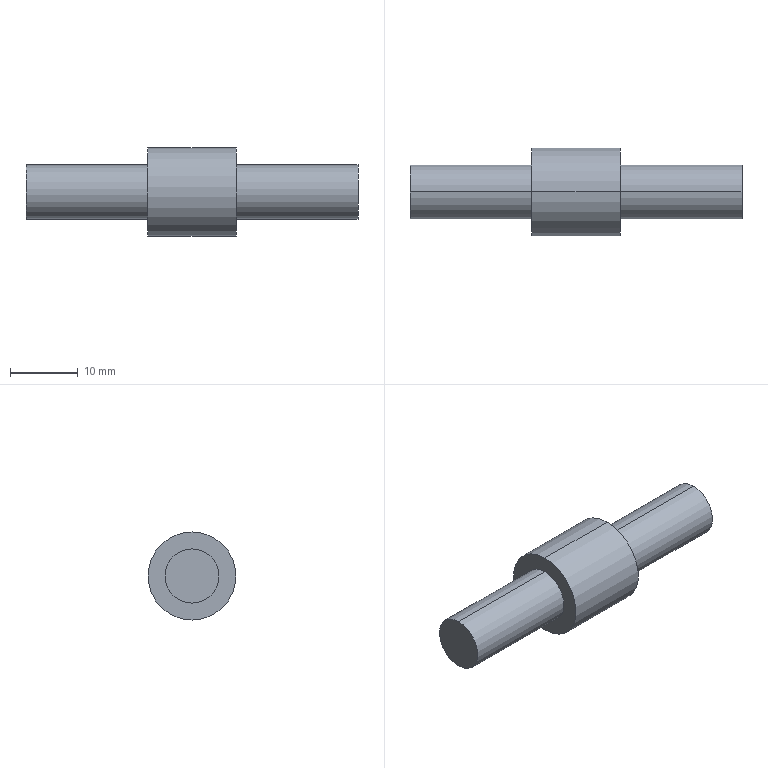Part | SolidWorks | features Extrusion 1, ICE 1, MirrorPattern 1 | 1 solid | 10 faces | box 49 x 13 x 13 mm | volume 3535 mm3 | cylinder 6 | plane 4 | commonest cylinder face diameters 8 x4 13 x2
STEP:
#1=CARTESIAN_POINT('',(-24.5,0.,-4.));
#2=VERTEX_POINT('',#1);
#3=CARTESIAN_POINT('',(-24.5,0.,4.));
#4=VERTEX_POINT('',#3);
#5=CARTESIAN_POINT('',(-24.5,0.,0.));
#6=DIRECTION('',(1.,0.,0.));
#7=DIRECTION('',(0.,0.,-1.));
#8=AXIS2_PLACEMENT_3D('',#5,#6,#7);
#9=CIRCLE('',#8,4.);
#10=EDGE_CURVE('',#2,#4,#9,.T.);
#11=ORIENTED_EDGE('',*,*,#10,.T.);
#12=CARTESIAN_POINT('',(-6.5,0.,4.));
#13=VERTEX_POINT('',#12);
#14=CARTESIAN_POINT('',(-24.5,0.,4.));
#15=DIRECTION('',(1.,0.,0.));
#16=VECTOR('',#15,1000.);
#17=LINE('',#14,#16);
#18=EDGE_CURVE('',#4,#13,#17,.T.);
#19=ORIENTED_EDGE('',*,*,#18,.T.);
#20=CARTESIAN_POINT('',(-6.5,0.,-4.));
#21=VERTEX_POINT('',#20);
#22=CARTESIAN_POINT('',(-6.5,0.,0.));
#23=DIRECTION('',(1.,0.,0.));
#24=DIRECTION('',(0.,0.,-1.));
#25=AXIS2_PLACEMENT_3D('',#22,#23,#24);
#26=CIRCLE('',#25,4.);
#27=EDGE_CURVE('',#21,#13,#26,.T.);
#28=ORIENTED_EDGE('',*,*,#27,.F.);
#29=CARTESIAN_POINT('',(-24.5,0.,-4.));
#30=DIRECTION('',(1.,0.,0.));
#31=VECTOR('',#30,1000.);
#32=LINE('',#29,#31);
#33=EDGE_CURVE('',#2,#21,#32,.T.);
#34=ORIENTED_EDGE('',*,*,#33,.F.);
#35=EDGE_LOOP('',(#11,#19,#28,#34));
#36=FACE_OUTER_BOUND('',#35,.T.);
#37=CARTESIAN_POINT('',(-24.5,0.,0.));
#38=DIRECTION('',(1.,0.,0.));
#39=DIRECTION('',(0.,0.,-1.));
#40=AXIS2_PLACEMENT_3D('',#37,#38,#39);
#41=CYLINDRICAL_SURFACE('',#40,4.);
#42=ADVANCED_FACE('',(#36),#41,.T.);
#43=CARTESIAN_POINT('',(24.5,0.,-4.));
#44=VERTEX_POINT('',#43);
#45=CARTESIAN_POINT('',(24.5,0.,4.));
#46=VERTEX_POINT('',#45);
#47=CARTESIAN_POINT('',(24.5,0.,0.));
#48=DIRECTION('',(1.,0.,0.));
#49=DIRECTION('',(0.,0.,-1.));
#50=AXIS2_PLACEMENT_3D('',#47,#48,#49);
#51=CIRCLE('',#50,4.);
#52=EDGE_CURVE('',#44,#46,#51,.T.);
#53=ORIENTED_EDGE('',*,*,#52,.F.);
#54=CARTESIAN_POINT('',(6.5,0.,-4.));
#55=VERTEX_POINT('',#54);
#56=CARTESIAN_POINT('',(24.5,0.,-4.));
#57=DIRECTION('',(-1.,0.,0.));
#58=VECTOR('',#57,1000.);
#59=LINE('',#56,#58);
#60=EDGE_CURVE('',#44,#55,#59,.T.);
#61=ORIENTED_EDGE('',*,*,#60,.T.);
#62=CARTESIAN_POINT('',(6.5,0.,4.));
#63=VERTEX_POINT('',#62);
#64=CARTESIAN_POINT('',(6.5,0.,0.));
#65=DIRECTION('',(1.,0.,0.));
#66=DIRECTION('',(0.,0.,-1.));
#67=AXIS2_PLACEMENT_3D('',#64,#65,#66);
#68=CIRCLE('',#67,4.);
#69=EDGE_CURVE('',#55,#63,#68,.T.);
#70=ORIENTED_EDGE('',*,*,#69,.T.);
#71=CARTESIAN_POINT('',(24.5,0.,4.));
#72=DIRECTION('',(-1.,0.,0.));
#73=VECTOR('',#72,1000.);
#74=LINE('',#71,#73);
#75=EDGE_CURVE('',#46,#63,#74,.T.);
#76=ORIENTED_EDGE('',*,*,#75,.F.);
#77=EDGE_LOOP('',(#53,#61,#70,#76));
#78=FACE_OUTER_BOUND('',#77,.T.);
#79=CARTESIAN_POINT('',(24.5,0.,0.));
#80=DIRECTION('',(-1.,0.,0.));
#81=DIRECTION('',(0.,0.,1.));
#82=AXIS2_PLACEMENT_3D('',#79,#80,#81);
#83=CYLINDRICAL_SURFACE('',#82,4.);
#84=ADVANCED_FACE('',(#78),#83,.T.);
#85=CARTESIAN_POINT('',(6.5,0.,-6.5));
#86=VERTEX_POINT('',#85);
#87=CARTESIAN_POINT('',(6.5,0.,6.5));
#88=VERTEX_POINT('',#87);
#89=CARTESIAN_POINT('',(6.5,0.,0.));
#90=DIRECTION('',(1.,0.,0.));
#91=DIRECTION('',(0.,0.,-1.));
#92=AXIS2_PLACEMENT_3D('',#89,#90,#91);
#93=CIRCLE('',#92,6.5);
#94=EDGE_CURVE('',#86,#88,#93,.T.);
#95=ORIENTED_EDGE('',*,*,#94,.F.);
#96=CARTESIAN_POINT('',(-6.5,0.,-6.5));
#97=VERTEX_POINT('',#96);
#98=CARTESIAN_POINT('',(6.5,0.,-6.5));
#99=DIRECTION('',(-1.,0.,0.));
#100=VECTOR('',#99,1000.);
#101=LINE('',#98,#100);
#102=EDGE_CURVE('',#86,#97,#101,.T.);
#103=ORIENTED_EDGE('',*,*,#102,.T.);
#104=CARTESIAN_POINT('',(-6.5,0.,6.5));
#105=VERTEX_POINT('',#104);
#106=CARTESIAN_POINT('',(-6.5,0.,0.));
#107=DIRECTION('',(1.,0.,0.));
#108=DIRECTION('',(0.,0.,-1.));
#109=AXIS2_PLACEMENT_3D('',#106,#107,#108);
#110=CIRCLE('',#109,6.5);
#111=EDGE_CURVE('',#97,#105,#110,.T.);
#112=ORIENTED_EDGE('',*,*,#111,.T.);
#113=CARTESIAN_POINT('',(6.5,0.,6.5));
#114=DIRECTION('',(-1.,0.,0.));
#115=VECTOR('',#114,1000.);
#116=LINE('',#113,#115);
#117=EDGE_CURVE('',#88,#105,#116,.T.);
#118=ORIENTED_EDGE('',*,*,#117,.F.);
#119=EDGE_LOOP('',(#95,#103,#112,#118));
#120=FACE_OUTER_BOUND('',#119,.T.);
#121=CARTESIAN_POINT('',(6.5,0.,0.));
#122=DIRECTION('',(-1.,0.,0.));
#123=DIRECTION('',(0.,0.,1.));
#124=AXIS2_PLACEMENT_3D('',#121,#122,#123);
#125=CYLINDRICAL_SURFACE('',#124,6.5);
#126=ADVANCED_FACE('',(#120),#125,.T.);
#127=ORIENTED_EDGE('',*,*,#102,.F.);
#128=CARTESIAN_POINT('',(6.5,0.,0.));
#129=DIRECTION('',(1.,0.,0.));
#130=DIRECTION('',(0.,0.,-1.));
#131=AXIS2_PLACEMENT_3D('',#128,#129,#130);
#132=CIRCLE('',#131,6.5);
#133=EDGE_CURVE('',#88,#86,#132,.T.);
#134=ORIENTED_EDGE('',*,*,#133,.F.);
#135=ORIENTED_EDGE('',*,*,#117,.T.);
#136=CARTESIAN_POINT('',(-6.5,0.,0.));
#137=DIRECTION('',(1.,0.,0.));
#138=DIRECTION('',(0.,0.,-1.));
#139=AXIS2_PLACEMENT_3D('',#136,#137,#138);
#140=CIRCLE('',#139,6.5);
#141=EDGE_CURVE('',#105,#97,#140,.T.);
#142=ORIENTED_EDGE('',*,*,#141,.T.);
#143=EDGE_LOOP('',(#127,#134,#135,#142));
#144=FACE_OUTER_BOUND('',#143,.T.);
#145=CARTESIAN_POINT('',(6.5,0.,0.));
#146=DIRECTION('',(-1.,0.,0.));
#147=DIRECTION('',(0.,0.,1.));
#148=AXIS2_PLACEMENT_3D('',#145,#146,#147);
#149=CYLINDRICAL_SURFACE('',#148,6.5);
#150=ADVANCED_FACE('',(#144),#149,.T.);
#151=CARTESIAN_POINT('',(6.5,0.,0.));
#152=DIRECTION('',(1.,0.,0.));
#153=DIRECTION('',(0.,0.,-1.));
#154=AXIS2_PLACEMENT_3D('',#151,#152,#153);
#155=CIRCLE('',#154,4.);
#156=EDGE_CURVE('',#63,#55,#155,.T.);
#157=ORIENTED_EDGE('',*,*,#156,.F.);
#158=ORIENTED_EDGE('',*,*,#69,.F.);
#159=EDGE_LOOP('',(#157,#158));
#160=FACE_BOUND('',#159,.T.);
#161=ORIENTED_EDGE('',*,*,#133,.T.);
#162=ORIENTED_EDGE('',*,*,#94,.T.);
#163=EDGE_LOOP('',(#161,#162));
#164=FACE_OUTER_BOUND('',#163,.T.);
#165=CARTESIAN_POINT('',(6.5,0.,0.));
#166=DIRECTION('',(1.,0.,0.));
#167=DIRECTION('',(0.,0.,-1.));
#168=AXIS2_PLACEMENT_3D('',#165,#166,#167);
#169=PLANE('',#168);
#170=ADVANCED_FACE('',(#160,#164),#169,.T.);
#171=ORIENTED_EDGE('',*,*,#27,.T.);
#172=CARTESIAN_POINT('',(-6.5,0.,0.));
#173=DIRECTION('',(1.,0.,0.));
#174=DIRECTION('',(0.,0.,-1.));
#175=AXIS2_PLACEMENT_3D('',#172,#173,#174);
#176=CIRCLE('',#175,4.);
#177=EDGE_CURVE('',#13,#21,#176,.T.);
#178=ORIENTED_EDGE('',*,*,#177,.T.);
#179=EDGE_LOOP('',(#171,#178));
#180=FACE_BOUND('',#179,.T.);
#181=ORIENTED_EDGE('',*,*,#141,.F.);
#182=ORIENTED_EDGE('',*,*,#111,.F.);
#183=EDGE_LOOP('',(#181,#182));
#184=FACE_OUTER_BOUND('',#183,.T.);
#185=CARTESIAN_POINT('',(-6.5,0.,0.));
#186=DIRECTION('',(1.,0.,0.));
#187=DIRECTION('',(0.,0.,-1.));
#188=AXIS2_PLACEMENT_3D('',#185,#186,#187);
#189=PLANE('',#188);
#190=ADVANCED_FACE('',(#180,#184),#189,.F.);
#191=ORIENTED_EDGE('',*,*,#60,.F.);
#192=CARTESIAN_POINT('',(24.5,0.,0.));
#193=DIRECTION('',(1.,0.,0.));
#194=DIRECTION('',(0.,0.,-1.));
#195=AXIS2_PLACEMENT_3D('',#192,#193,#194);
#196=CIRCLE('',#195,4.);
#197=EDGE_CURVE('',#46,#44,#196,.T.);
#198=ORIENTED_EDGE('',*,*,#197,.F.);
#199=ORIENTED_EDGE('',*,*,#75,.T.);
#200=ORIENTED_EDGE('',*,*,#156,.T.);
#201=EDGE_LOOP('',(#191,#198,#199,#200));
#202=FACE_OUTER_BOUND('',#201,.T.);
#203=CARTESIAN_POINT('',(24.5,0.,0.));
#204=DIRECTION('',(-1.,0.,0.));
#205=DIRECTION('',(0.,0.,1.));
#206=AXIS2_PLACEMENT_3D('',#203,#204,#205);
#207=CYLINDRICAL_SURFACE('',#206,4.);
#208=ADVANCED_FACE('',(#202),#207,.T.);
#209=ORIENTED_EDGE('',*,*,#197,.T.);
#210=ORIENTED_EDGE('',*,*,#52,.T.);
#211=EDGE_LOOP('',(#209,#210));
#212=FACE_OUTER_BOUND('',#211,.T.);
#213=CARTESIAN_POINT('',(24.5,0.,0.));
#214=DIRECTION('',(1.,0.,0.));
#215=DIRECTION('',(0.,0.,-1.));
#216=AXIS2_PLACEMENT_3D('',#213,#214,#215);
#217=PLANE('',#216);
#218=ADVANCED_FACE('',(#212),#217,.T.);
#219=ORIENTED_EDGE('',*,*,#18,.F.);
#220=CARTESIAN_POINT('',(-24.5,0.,0.));
#221=DIRECTION('',(1.,0.,0.));
#222=DIRECTION('',(0.,0.,-1.));
#223=AXIS2_PLACEMENT_3D('',#220,#221,#222);
#224=CIRCLE('',#223,4.);
#225=EDGE_CURVE('',#4,#2,#224,.T.);
#226=ORIENTED_EDGE('',*,*,#225,.T.);
#227=ORIENTED_EDGE('',*,*,#33,.T.);
#228=ORIENTED_EDGE('',*,*,#177,.F.);
#229=EDGE_LOOP('',(#219,#226,#227,#228));
#230=FACE_OUTER_BOUND('',#229,.T.);
#231=CARTESIAN_POINT('',(-24.5,0.,0.));
#232=DIRECTION('',(1.,0.,0.));
#233=DIRECTION('',(0.,0.,-1.));
#234=AXIS2_PLACEMENT_3D('',#231,#232,#233);
#235=CYLINDRICAL_SURFACE('',#234,4.);
#236=ADVANCED_FACE('',(#230),#235,.T.);
#237=ORIENTED_EDGE('',*,*,#10,.F.);
#238=ORIENTED_EDGE('',*,*,#225,.F.);
#239=EDGE_LOOP('',(#237,#238));
#240=FACE_OUTER_BOUND('',#239,.T.);
#241=CARTESIAN_POINT('',(-24.5,0.,0.));
#242=DIRECTION('',(-1.,0.,0.));
#243=DIRECTION('',(0.,0.,-1.));
#244=AXIS2_PLACEMENT_3D('',#241,#242,#243);
#245=PLANE('',#244);
#246=ADVANCED_FACE('',(#240),#245,.T.);
#247=CLOSED_SHELL('',(#42,#84,#126,#150,#170,#190,#208,#218,#236,#246));
#248=MANIFOLD_SOLID_BREP('',#247);
#249=CARTESIAN_POINT('',(0.,0.,0.));
#250=DIRECTION('',(0.,0.,1.));
#251=DIRECTION('',(1.,0.,0.));
#252=AXIS2_PLACEMENT_3D('',#249,#250,#251);
#253=(LENGTH_UNIT()NAMED_UNIT(*)SI_UNIT(.MILLI.,.METRE.));
#254=UNCERTAINTY_MEASURE_WITH_UNIT(LENGTH_MEASURE(0.00001),#253,'','');
#255=(NAMED_UNIT(*)PLANE_ANGLE_UNIT()SI_UNIT($,.RADIAN.));
#256=(NAMED_UNIT(*)SI_UNIT($,.STERADIAN.)SOLID_ANGLE_UNIT());
#257=(GEOMETRIC_REPRESENTATION_CONTEXT(3)GLOBAL_UNCERTAINTY_ASSIGNED_CONTEXT((#254))GLOBAL_UNIT_ASSIGNED_CONTEXT((#253,#255,#256))REPRESENTATION_CONTEXT('',''));
#258=ADVANCED_BREP_SHAPE_REPRESENTATION('',(#248,#252),#257);